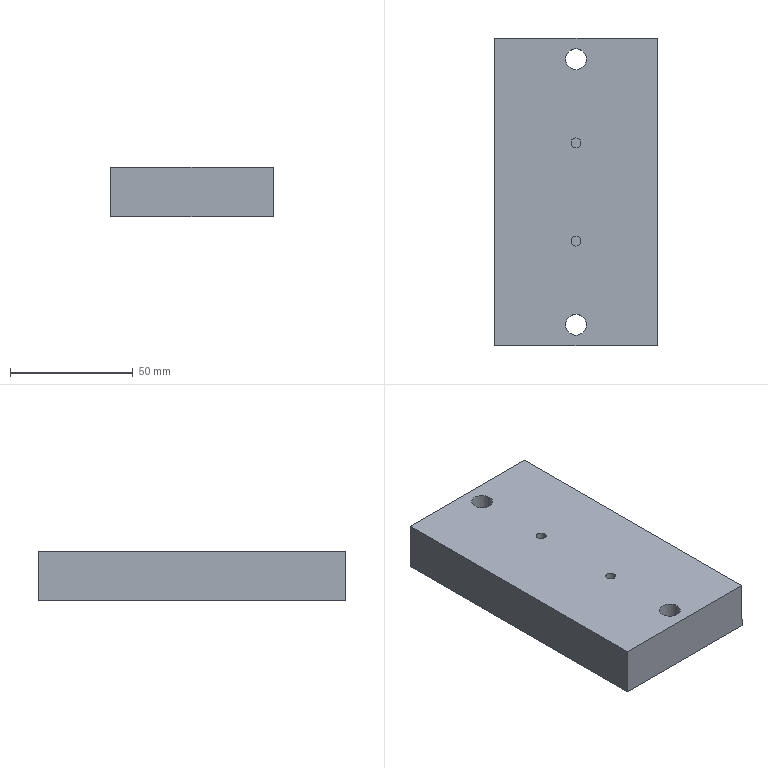NC program | NX | posted with a generic post | part box 65.936 x 125 x 20 mm
Lines 1 to 1208 of 29196:
N10 G17 G21 G94 G90
(FACE_MILLING , TOOL : D63)
N12 T01 M6
N14 G54
N16 G17 G0 G90 X86.95 Y-24.269 S4000 M3
N18 G43 Z33. H1
N20 G94 G1 Z0. F5000.
N22 X77.5 F1200.
N24 X-77.5
N26 Y24.269
N28 X77.5
N30 X86.95
N32 G0 Z33.
(FLOOR_WALL , TOOL : D63)
N34 X82.5 Y-2.101
N36 Z30.
N38 G1 Z-1.852 F5000.
N40 X74.5 F1500.
N42 X-74.5
N44 Y2.507
N46 X74.5
N48 X82.5
N50 G0 Y-2.101 Z-3.277
N52 G1 X74.5
N54 X-74.5
N56 Y2.507
N58 X74.5
N60 X82.5
N62 G0 Z30.
(FLOOR_WALL_COPY , TOOL : D63)
N64 Y-1.542
N66 G1 Z-3.427 F5000.
N68 X74.5 F1200.
N70 X-74.5
N72 Y2.402
N74 X74.5
N76 X82.5
N78 G0 Z30.
N80 M5
(PLANAR_MILL , TOOL : D16R0波刀)
N82 T02 M6
N84 G54
N86 G17 G0 G90 X-57.998 Y49.656 S5500 M3
N88 G43 Z30. H2
N90 G94 G1 Z-2.5 F5000.
N92 X-45.998 F2000.
N94 X54.35
N96 Y-41.952
N98 X46.374 Y-49.656
N100 X-46.374
N102 X-54.35 Y-41.952
N104 Y36.799
N106 Y48.799
N108 G0 X-57.998 Y49.656 Z-5.
N110 G1 X-45.998
N112 X54.35
N114 Y-41.952
N116 X46.374 Y-49.656
N118 X-46.374
N120 X-54.35 Y-41.952
N122 Y36.799
N124 Y48.799
N126 G0 X-57.998 Y49.656 Z-7.5
N128 G1 X-45.998
N130 X54.35
N132 Y-41.952
N134 X46.374 Y-49.656
N136 X-46.374
N138 X-54.35 Y-41.952
N140 Y36.799
N142 Y48.799
N144 G0 X-57.998 Y49.656 Z-10.
N146 G1 X-45.998
N148 X54.35
N150 Y-41.952
N152 X46.374 Y-49.656
N154 X-46.374
N156 X-54.35 Y-41.952
N158 Y36.799
N160 Y48.799
N162 G0 X-57.998 Y49.656 Z-12.5
N164 G1 X-45.998
N166 X54.35
N168 Y-41.952
N170 X46.374 Y-49.656
N172 X-46.374
N174 X-54.35 Y-41.952
N176 Y36.799
N178 Y48.799
N180 G0 X-57.998 Y49.656 Z-15.
N182 G1 X-45.998
N184 X54.35
N186 Y-41.952
N188 X46.374 Y-49.656
N190 X-46.374
N192 X-54.35 Y-41.952
N194 Y36.799
N196 Y48.799
N198 G0 X-57.998 Y49.656 Z-17.5
N200 G1 X-45.998
N202 X54.35
N204 Y-41.952
N206 X46.374 Y-49.656
N208 X-46.374
N210 X-54.35 Y-41.952
N212 Y36.799
N214 Y48.799
N216 G0 X-57.998 Y49.656 Z-20.
N218 G1 X-45.998
N220 X54.35
N222 Y-41.952
N224 X46.374 Y-49.656
N226 X-46.374
N228 X-54.35 Y-41.952
N230 Y36.799
N232 Y48.799
N234 G0 X-57.998 Y49.656 Z-22.5
N236 G1 X-45.998
N238 X54.35
N240 Y-41.952
N242 X46.374 Y-49.656
N244 X-46.374
N246 X-54.35 Y-41.952
N248 Y36.799
N250 Y48.799
N252 G0 X-57.998 Y49.656 Z-25.
N254 G1 X-45.998
N256 X54.35
N258 Y-41.952
N260 X46.374 Y-49.656
N262 X-46.374
N264 X-54.35 Y-41.952
N266 Y36.799
N268 Y48.799
N270 G0 X-57.998 Y49.656 Z-27.5
N272 G1 X-45.998
N274 X54.35
N276 Y-41.952
N278 X46.374 Y-49.656
N280 X-46.374
N282 X-54.35 Y-41.952
N284 Y36.799
N286 Y48.799
N288 G0 X-57.998 Y49.656 Z-28.352
N290 G1 X-45.998
N292 X54.35
N294 Y-41.952
N296 X46.374 Y-49.656
N298 X-46.374
N300 X-54.35 Y-41.952
N302 Y36.799
N304 Y48.799
N306 G0 Z30.
(PLANAR_MILL_COPY , TOOL : D16R0波刀)
N308 Z30.
N310 X58. Y-37.306
N312 G1 Z-2.335 F5000.
N314 X46. F2000.
N316 X-46.
N318 X-58.
N320 G0 Z30.
(ZLEVEL_PROFILE , TOOL : D16R0波刀)
N322 Z30.5
N324 X-56.72 Y45.12
N326 G1 Z0.203 F5000.
N328 X-46.32 F4000.
N330 X46.32
N332 X56.72
N334 G0 X56.871 Y45.544 Z-0.094
N336 G1 X46.471
N338 X-46.471
N340 X-56.871
N342 G0 Y45.967 Z-0.39
N344 G1 X-46.471
N346 X46.471
N348 X56.871
N350 G0 Y46.325 Z-0.687
N352 G1 X46.472 Y46.391
N354 X46.419
N356 X-46.472
N358 X-56.872
N360 G0 X-56.873 Y46.815 Z-0.984
N362 G1 X-46.473
N364 X46.421
N366 X46.473
N368 X56.872 Y46.751
N370 G0 Y47.184 Z-1.281
N372 G1 X46.473 Y47.239
N374 X46.429
N376 X-46.473
N378 X-56.873
N380 G0 X-56.872 Y47.663 Z-1.577
N382 G1 X-46.472
N384 X46.428
N386 X46.472 Y47.662
N388 X56.872 Y47.607
N390 G0 Y48.056 Z-1.874
N392 G1 X46.472 Y48.086
N394 X46.447
N396 X-46.472 Y48.087
N398 X-56.872
N400 G0 X-56.871 Y48.51 Z-2.171
N402 G1 X-46.471
N404 X46.471
N406 X56.871
N408 G0 Y48.934 Z-2.468
N410 G1 X46.471
N412 X-46.471
N414 X-56.871
N416 G0 X-56.682 Y49.358 Z-2.764
N418 G1 X-46.282
N420 X46.282
N422 X56.682
N424 G0 X56.299 Y49.782 Z-3.061
N426 G1 X45.899
N428 X-45.899
N430 X-56.299
N432 G0 Z30.5
(ZLEVEL_PROFILE_COPY_COPY_COPY , TOOL : D16R0波刀)
N434 X56.484 Y28.517
N436 Z30.5
N438 G1 Z0.205 F5000.
N440 X46.084 F4000.
N442 X-46.084
N444 X-56.484
N446 G0 X-56.705 Y28.323 Z-0.09
N448 G1 X-46.305 Y28.311
N450 X-45.799 Y28.31
N452 X45.799
N454 X46.305 Y28.311
N456 X56.705 Y28.323
N458 G0 X56.871 Y28.116 Z-0.385
N460 G1 X46.471 Y28.104
N462 X45.761
N464 X-46.471
N466 X-56.871
N468 G0 Y27.897 Z-0.681
N470 G1 X-46.471
N472 X45.761
N474 X46.471 Y27.898
N476 X56.871 Y27.909
N478 G0 X56.888 Y27.69 Z-0.976
N480 G1 X46.488
N482 X-46.471
N484 X-56.871
N486 G0 Y27.484 Z-1.271
N488 G1 X-46.471
N490 X45.761
N492 X46.471
N494 X56.871 Y27.496
N496 G0 X56.899 Y27.277 Z-1.566
N498 G1 X46.499
N500 X-46.47
N502 X-56.871
N504 G0 Y27.071 Z-1.861
N506 G1 X-46.471 Y27.07
N508 X45.761
N510 X46.471 Y27.071
N512 X56.871 Y27.082
N514 G0 X56.899 Y26.864 Z-2.156
N516 G1 X46.499
N518 X-46.467
N520 X-46.471
N522 X-56.871 Y26.868
N524 G0 Y26.662 Z-2.451
N526 G1 X-46.471 Y26.657
N528 X-46.467
N530 X46.504
N532 X56.904
N534 G0 X56.902 Y26.45 Z-2.747
N536 G1 X46.502
N538 X-46.465
N540 X-56.865
N542 G0 X-56.561 Y26.256 Z-3.042
N544 G1 X-46.161 Y26.244
N546 X-45.799
N548 X45.799
N550 X46.161
N552 X56.561 Y26.256
N554 G0 X56.374 Y26.038 Z-3.337
N556 G1 X45.974
N558 X-45.974
N560 X-56.374
N562 G0 Z30.5
(ZLEVEL_PROFILE_COPY , TOOL : D16R0波刀)
N564 X56.709 Y-45.181
N566 Z27.965
N568 G1 Z-2.313 F5000.
N570 X46.309 F4000.
N572 X-46.309
N574 X-56.709
N576 G0 X-56.871 Y-45.63 Z-2.592
N578 G1 X-46.471 Y-45.663
N580 X-46.445
N582 X46.471
N584 X56.871
N586 G0 Y-46.146 Z-2.871
N588 G1 X46.471
N590 X-46.422
N592 X-46.471 Y-46.145
N594 X-56.871 Y-46.084
N596 G0 Y-46.595 Z-3.149
N598 G1 X-46.471 Y-46.628
N600 X-46.445
N602 X46.471
N604 X56.871
N606 G0 Y-47.111 Z-3.428
N608 G1 X46.471
N610 X-46.445
N612 X-46.471
N614 X-56.871 Y-47.078
N616 G0 Y-47.593 Z-3.706
N618 G1 X-46.471
N620 X46.471
N622 X56.871
N624 G0 Y-48.076 Z-3.985
N626 G1 X46.471
N628 X-46.464
N630 X-46.471
N632 X-56.871 Y-48.067
N634 G0 Y-48.492 Z-4.263
N636 G1 X-46.471 Y-48.558
N638 X-46.419
N640 X46.471
N642 X56.871
N644 G0 Y-49.041 Z-4.542
N646 G1 X46.471
N648 X-46.471
N650 X-56.871
N652 G0 X-56.618 Y-49.523 Z-4.821
N654 G1 X-46.218
N656 X46.218
N658 X56.618
N660 G0 Z27.965
(ZLEVEL_PROFILE_COPY_COPY , TOOL : D16R0波刀)
N662 X-56.871 Y-28.436
N664 G1 Z-2.305 F5000.
N666 X-46.471 Y-28.371 F3000.
N668 X-46.42
N670 X46.42
N672 X46.471
N674 X56.871 Y-28.436
N676 G0 X56.872 Y-27.362 Z-2.576
N678 G1 X46.472
N680 X-46.472
N682 X-56.872
N684 G0 X-56.871 Y-26.411 Z-2.846
N686 G1 X-46.471 Y-26.353
N688 X-46.426
N690 X46.426
N692 X46.471
N694 X56.871 Y-26.411
N696 G0 X56.517 Y-25.356 Z-3.116
N698 G1 X46.117 Y-25.344
N700 X45.799 Y-25.343
N702 X-45.799
N704 X-46.117 Y-25.344
N706 X-56.517 Y-25.356
N708 G0 Z27.965
N710 M5
(PLANAR_MILL_COPY_COPY , TOOL : D8R0)
N712 T03 M6
N714 G54
N716 G17 G0 G90 X51.2 Y30.401 S4500 M3
N718 G43 Z26.583 H3
N720 G94 G1 Z-3.417 F5000.
N722 X46. F1000.
N724 X-46.
N726 X-51.2
N728 G0 Z26.583
N730 Y-29.535
N732 G1 Z-3.417 F5000.
N734 X-46. F1000.
N736 X46.
N738 X51.2
N740 G0 Z26.583
(PLANAR_MILL_COPY_2 , TOOL : D8R0)
N742 Z30.
N744 X-51.999 Y45.306
N746 G1 Z-15. F5000.
N748 X-45.999 F800.
N750 X50.
N752 Y-40.106
N754 X44.616 Y-45.306
N756 X-44.616
N758 X-50. Y-40.106
N760 Y36.799
N762 Y43.999
N764 G0 X-51.999 Y45.306 Z-28.352
N766 G1 X-45.999
N768 X50.
N770 Y-40.106
N772 X44.616 Y-45.306
N774 X-44.616
N776 X-50. Y-40.106
N778 Y36.799
N780 Y43.999
N782 G0 Z30.
N784 M5
(FIXED_CONTOUR , TOOL : D4R0.5)
N786 T04 M6
N788 G54
N790 G17 G0 G90 X-48. Y40.587 S6000 M3
N792 G43 Z30. H4
N794 G94 G1 Z-0.09 F5000.
N796 G3 X-46. Y38.587 R2. F3000.
N798 G1 X46.
N800 Y38.663 Z-0.143
N802 X-46.
N804 Y38.738 Z-0.196
N806 X46.
N808 Y38.813 Z-0.248
N810 X-46.
N812 Y38.888 Z-0.301
N814 X46.
N816 Y38.963 Z-0.353
N818 X-46.
N820 Y39.038 Z-0.406
N822 X46.
N824 Y39.113 Z-0.458
N826 X-46.
N828 Y39.188 Z-0.511
N830 X46.
N832 Y39.263 Z-0.564
N834 X-46.
N836 Y39.338 Z-0.616
N838 X46.
N840 Y39.413 Z-0.669
N842 X-46.
N844 Y39.489 Z-0.721
N846 X46.
N848 Y39.564 Z-0.774
N850 X-46.
N852 Y39.639 Z-0.827
N854 X46.
N856 Y39.714 Z-0.879
N858 X-46.
N860 Y39.789 Z-0.932
N862 X46.
N864 Y39.864 Z-0.984
N866 X-46.
N868 Y39.939 Z-1.037
N870 X46.
N872 Y40.014 Z-1.089
N874 X-46.
N876 Y40.089 Z-1.142
N878 X46.
N880 Y40.164 Z-1.195
N882 X-46.
N884 Y40.239 Z-1.247
N886 X46.
N888 Y40.314 Z-1.3
N890 X-46.
N892 Y40.39 Z-1.352
N894 X46.
N896 Y40.465 Z-1.405
N898 X-46.
N900 Y40.54 Z-1.457
N902 X46.
N904 Y40.615 Z-1.51
N906 X-46.
N908 Y40.69 Z-1.563
N910 X46.
N912 Y40.765 Z-1.615
N914 X-46.
N916 Y40.84 Z-1.668
N918 X46.
N920 Y40.915 Z-1.72
N922 X-46.
N924 Y40.99 Z-1.773
N926 X46.
N928 Y41.065 Z-1.825
N930 X-46.
N932 Y41.14 Z-1.878
N934 X46.
N936 Y41.216 Z-1.931
N938 X-46.
N940 Y41.291 Z-1.983
N942 X46.
N944 Y41.366 Z-2.036
N946 X-46.
N948 Y41.441 Z-2.088
N950 X46.
N952 Y41.516 Z-2.141
N954 X-46.
N956 Y41.591 Z-2.194
N958 X46.
N960 Y41.666 Z-2.246
N962 X-46.
N964 Y41.741 Z-2.299
N966 X46.
N968 Y41.816 Z-2.351
N970 X-46.
N972 Y41.891 Z-2.404
N974 X46.
N976 Y41.966 Z-2.456
N978 X-46.
N980 Y42.042 Z-2.509
N982 X46.
N984 Y42.117 Z-2.562
N986 X-46.
N988 Y42.192 Z-2.614
N990 X46.
N992 Y42.267 Z-2.667
N994 X-46.
N996 Y42.342 Z-2.719
N998 X46.
N1000 Y42.417 Z-2.772
N1002 X-46.
N1004 Y42.492 Z-2.824
N1006 X46.
N1008 Y42.567 Z-2.877
N1010 X-46.
N1012 Y42.642 Z-2.93
N1014 X46.
N1016 Y42.717 Z-2.982
N1018 X-46.
N1020 Y42.792 Z-3.035
N1022 X46.
N1024 Y42.868 Z-3.087
N1026 X-46.
N1028 Y42.943 Z-3.14
N1030 X46.
N1032 Y43.018 Z-3.193
N1034 X-46.
N1036 Y43.093 Z-3.245
N1038 X46.
N1040 G3 X48. Y45.093 R2.
N1042 G0 Z30.
(ZLEVEL_PROFILE_1 , TOOL : D4R0.5)
N1044 X48.6 Y34.874
N1046 G1 Z-0.237 F5000.
N1048 X46. F2500.
N1050 X-46.
N1052 X-48.6
N1054 G0 Y34.819 Z-0.316
N1056 G1 X-46.
N1058 X46.
N1060 X48.6
N1062 G0 Y34.764 Z-0.395
N1064 G1 X46.
N1066 X-46.
N1068 X-48.6
N1070 G0 Y34.708 Z-0.474
N1072 G1 X-46.
N1074 X46.
N1076 X48.6
N1078 G0 Y34.653 Z-0.553
N1080 G1 X46.
N1082 X-46.
N1084 X-48.6
N1086 G0 Y34.597 Z-0.633
N1088 G1 X-46.
N1090 X46.
N1092 X48.6
N1094 G0 Y34.542 Z-0.712
N1096 G1 X46.
N1098 X-46.
N1100 X-48.6
N1102 G0 Y34.487 Z-0.791
N1104 G1 X-46.
N1106 X46.
N1108 X48.6
N1110 G0 Y34.431 Z-0.87
N1112 G1 X46.
N1114 X-46.
N1116 X-48.6
N1118 G0 Y34.376 Z-0.949
N1120 G1 X-46.
N1122 X46.
N1124 X48.6
N1126 G0 Y34.321 Z-1.028
N1128 G1 X46.
N1130 X-46.
N1132 X-48.6
N1134 G0 Y34.265 Z-1.107
N1136 G1 X-46.
N1138 X46.
N1140 X48.6
N1142 G0 Y34.21 Z-1.186
N1144 G1 X46.
N1146 X-46.
N1148 X-48.6
N1150 G0 Y34.155 Z-1.265
N1152 G1 X-46.
N1154 X46.
N1156 X48.6
N1158 G0 Y34.099 Z-1.344
N1160 G1 X46.
N1162 X-46.
N1164 X-48.6
N1166 G0 Y34.044 Z-1.423
N1168 G1 X-46.
N1170 X46.
N1172 X48.6
N1174 G0 Y33.988 Z-1.502
N1176 G1 X46.
N1178 X-46.
N1180 X-48.6
N1182 G0 Y33.933 Z-1.581
N1184 G1 X-46.
N1186 X46.
N1188 X48.6
N1190 G0 Y33.878 Z-1.66
N1192 G1 X46.
N1194 X-46.
N1196 X-48.6
N1198 G0 Y33.822 Z-1.74
N1200 G1 X-46.
N1202 X46.
N1204 X48.6
N1206 G0 Y33.767 Z-1.819
N1208 G1 X46.
N1210 X-46.
N1212 X-48.6
N1214 G0 Y33.712 Z-1.898
N1216 G1 X-46.
N1218 X46.
N1220 X48.6
N1222 G0 Y33.656 Z-1.977
N1224 G1 X46.
N1226 X-46.
N1228 X-48.6
N1230 G0 Y33.601 Z-2.056
N1232 G1 X-46.
N1234 X46.
N1236 X48.6
N1238 G0 Y33.546 Z-2.135
N1240 G1 X46.
N1242 X-46.
N1244 X-48.6
N1246 G0 Y33.49 Z-2.214
N1248 G1 X-46.
N1250 X46.
N1252 X48.6
N1254 G0 Y33.435 Z-2.293
N1256 G1 X46.
N1258 X-46.
N1260 X-48.6
N1262 G0 Y33.379 Z-2.372
N1264 G1 X-46.
N1266 X46.
N1268 X48.6
N1270 G0 Y33.324 Z-2.451
N1272 G1 X46.
N1274 X-46.
N1276 X-48.6
N1278 G0 Y33.269 Z-2.53
N1280 G1 X-46.
N1282 X46.
N1284 X48.6
N1286 G0 Y33.213 Z-2.609
N1288 G1 X46.
N1290 X-46.
N1292 X-48.6
N1294 G0 Y33.158 Z-2.688
N1296 G1 X-46.
N1298 X46.
N1300 X48.6
N1302 G0 Y33.103 Z-2.767
N1304 G1 X46.
N1306 X-46.
N1308 X-48.6
N1310 G0 Y33.047 Z-2.847
N1312 G1 X-46.
N1314 X46.
N1316 X48.6
N1318 G0 Y32.992 Z-2.926
N1320 G1 X46.
N1322 X-46.
N1324 X-48.6
N1326 G0 Y32.936 Z-3.005
N1328 G1 X-46.
N1330 X46.
N1332 X48.6
N1334 G0 Y32.881 Z-3.084
N1336 G1 X46.
N1338 X-46.
N1340 X-48.6
N1342 G0 Y32.826 Z-3.163
N1344 G1 X-46.
N1346 X46.
N1348 X48.6
N1350 G0 Y32.77 Z-3.242
N1352 G1 X46.
N1354 X-46.
N1356 X-48.6
N1358 G0 Y32.715 Z-3.321
N1360 G1 X-46.
N1362 X46.
N1364 X48.6
N1366 G0 Y32.66 Z-3.4
N1368 G1 X46.
N1370 X-46.
N1372 X-48.6
N1374 G0 Z30.
(ZLEVEL_PROFILE_1_COPY , TOOL : D4R0.5)
N1376 X-48.653 Y-35.529
N1378 Z27.665
N1380 G1 Z-2.515 F5000.
N1382 X-46.057 Y-35.378 F2000.
N1384 X-45.987 Y-35.374
N1386 X45.987
N1388 X46.057 Y-35.378
N1390 X48.653 Y-35.529
N1392 G0 X48.785 Y-35.3 Z-2.535
N1394 G1 X46.185 Y-35.299
N1396 X45.987
N1398 X-46.185
N1400 X-48.785
N1402 G0 Y-35.225 Z-2.555
N1404 G1 X-46.185
N1406 X45.987
N1408 X46.185
N1410 X48.785
N1412 G0 Y-35.211 Z-2.575
N1414 G1 X46.185 Y-35.151
N1416 X46.144 Y-35.15
N1418 X-46.146
N1420 X-46.185
N1422 X-48.785 Y-35.209
N1424 G0 Y-35.075 Z-2.595
N1426 G1 X-46.185
N1428 X45.987
N1430 X46.185
N1432 X48.785
N1434 G0 Y-35.001 Z-2.615
N1436 G1 X46.185
N1438 X-46.185
N1440 X-48.785
N1442 G0 Y-34.926 Z-2.635
N1444 G1 X-46.185
N1446 X46.185
N1448 X48.785
N1450 G0 Y-34.883 Z-2.655
N1452 G1 X46.185 Y-34.852
N1454 X46.165 Y-34.851
N1456 X-46.164
N1458 X-46.185 Y-34.852
N1460 X-48.785 Y-34.883
N1462 G0 Y-34.777 Z-2.675
N1464 G1 X-46.185
N1466 X46.159
N1468 X46.185
N1470 X48.785 Y-34.816
N1472 G0 Y-34.761 Z-2.695
N1474 G1 X46.185 Y-34.703
N1476 X46.146 Y-34.702
N1478 X-46.146
N1480 X-46.185 Y-34.703
N1482 X-48.785 Y-34.761
N1484 G0 Y-34.687 Z-2.715
N1486 G1 X-46.185 Y-34.628
N1488 X-46.145
N1490 X46.145
N1492 X46.185
N1494 X48.785 Y-34.688
N1496 G0 Y-34.611 Z-2.735
N1498 G1 X46.185 Y-34.553
N1500 X46.146
N1502 X-46.146
N1504 X-46.185
N1506 X-48.785 Y-34.611
N1508 G0 Y-34.541 Z-2.755
N1510 G1 X-46.185 Y-34.479
N1512 X-46.143 Y-34.478
N1514 X46.144
N1516 X46.185 Y-34.479
N1518 X48.785 Y-34.54
N1520 G0 Y-34.463 Z-2.775
N1522 G1 X46.185 Y-34.404
N1524 X46.145
N1526 X-46.146
N1528 X-46.185
N1530 X-48.785 Y-34.462
N1532 G0 Y-34.387 Z-2.795
N1534 G1 X-46.185 Y-34.329
N1536 X-46.146
N1538 X46.147
N1540 X46.185
N1542 X48.785 Y-34.386
N1544 G0 Y-34.254 Z-2.815
N1546 G1 X46.185
N1548 X-46.185
N1550 X-48.785 Y-34.255
N1552 G0 Y-34.18 Z-2.835
N1554 G1 X-46.185
N1556 X46.185
N1558 X48.785
N1560 G0 Y-34.105 Z-2.855
N1562 G1 X46.185
N1564 X-46.185
N1566 X-48.785
N1568 G0 X-48.786 Y-34.03 Z-2.875
N1570 G1 X-46.186
N1572 X46.186
N1574 X48.786
N1576 G0 Y-33.956 Z-2.895
N1578 G1 X46.186
N1580 X-46.186
N1582 X-48.786
N1584 G0 Y-33.881 Z-2.915
N1586 G1 X-46.186
N1588 X46.186
N1590 X48.786
N1592 G0 Y-33.806 Z-2.935
N1594 G1 X46.186
N1596 X-46.186
N1598 X-48.786
N1600 G0 Y-33.732 Z-2.955
N1602 G1 X-46.186
N1604 X46.186
N1606 X48.786
N1608 G0 Y-33.657 Z-2.975
N1610 G1 X46.186
N1612 X-46.186
N1614 X-48.786
N1616 G0 Y-33.583 Z-2.995
N1618 G1 X-46.186
N1620 X46.186
N1622 X48.786
N1624 G0 Y-33.508 Z-3.015
N1626 G1 X46.186
N1628 X-46.186 Y-33.52
N1630 X-48.786
N1632 G0 Y-33.494 Z-3.035
N1634 G1 X-46.186 Y-33.434
N1636 X-46.145 Y-33.433
N1638 X46.146
N1640 X46.186 Y-33.434
N1642 X48.786 Y-33.493
N1644 G0 Y-33.416 Z-3.055
N1646 G1 X46.186 Y-33.359
N1648 X46.148
N1650 X-46.148
N1652 X-46.186
N1654 X-48.786 Y-33.416
N1656 G0 Y-33.346 Z-3.075
N1658 G1 X-46.186 Y-33.285
N1660 X-46.144 Y-33.284
N1662 X46.144
N1664 X46.186 Y-33.285
N1666 X48.785 Y-33.346
N1668 G0 X48.786 Y-33.269 Z-3.095
N1670 G1 X46.186 Y-33.21
N1672 X46.146 Y-33.209
N1674 X-46.146
N1676 X-46.186 Y-33.21
N1678 X-48.786 Y-33.269
N1680 G0 Y-33.192 Z-3.115
N1682 G1 X-46.186 Y-33.135
N1684 X-46.147
N1686 X46.147
N1688 X46.186
N1690 X48.786 Y-33.193
N1692 G0 X48.785 Y-33.121 Z-3.135
N1694 G1 X46.186 Y-33.061
N1696 X46.145 Y-33.06
N1698 X-46.146
N1700 X-46.186 Y-33.061
N1702 X-48.785 Y-33.12
N1704 G0 X-48.786 Y-32.985 Z-3.155
N1706 G1 X-46.186
N1708 X46.146
N1710 X46.186 Y-32.986
N1712 X48.785 Y-33.044
N1714 G0 Y-32.911 Z-3.175
N1716 G1 X46.185
N1718 X-46.185
N1720 X-48.785
N1722 G0 Y-32.836 Z-3.195
N1724 G1 X-46.185
N1726 X46.185
N1728 X48.785
N1730 G0 Y-32.762 Z-3.215
N1732 G1 X46.185
N1734 X-46.185
N1736 X-48.785
N1738 G0 Y-32.687 Z-3.235
N1740 G1 X-46.185
N1742 X46.185
N1744 X48.785
N1746 G0 Y-32.612 Z-3.255
N1748 G1 X46.185
N1750 X-46.185
N1752 X-48.785
N1754 G0 Y-32.538 Z-3.275
N1756 G1 X-46.185
N1758 X46.185
N1760 X48.785
N1762 G0 Y-32.497 Z-3.295
N1764 G1 X46.185 Y-32.463
N1766 X46.163
N1768 X-46.163
N1770 X-46.185
N1772 X-48.785 Y-32.497
N1774 G0 Y-32.388 Z-3.315
N1776 G1 X-46.185
N1778 X46.185
N1780 X48.785
N1782 G0 Y-32.314 Z-3.335
N1784 G1 X46.185
N1786 X-46.185
N1788 X-48.785
N1790 G0 Y-32.298 Z-3.355
N1792 G1 X-46.185 Y-32.239
N1794 X-46.145
N1796 X46.185
N1798 X48.785
N1800 G0 Y-32.19 Z-3.375
N1802 G1 X46.185 Y-32.164
N1804 X46.169
N1806 X-46.185
N1808 X-48.785
N1810 G0 Y-32.09 Z-3.395
N1812 G1 X-46.185
N1814 X46.185
N1816 X48.785
N1818 G0 Z27.665
(FIXED_CONTOUR_COPY , TOOL : D4R0.5)
N1820 X-48. Y-40.615
N1822 Z27.465
N1824 G1 Z-2.602 F5000.
N1826 G2 X-46. Y-38.615 R2. F2500.
N1828 G1 X46.
N1830 Y-38.706 Z-2.654
N1832 X-46.
N1834 Y-38.797 Z-2.707
N1836 X46.
N1838 Y-38.888 Z-2.759
N1840 X-46.
N1842 Y-38.978 Z-2.812
N1844 X46.
N1846 Y-39.069 Z-2.864
N1848 X-46.
N1850 Y-39.16 Z-2.916
N1852 X46.
N1854 Y-39.251 Z-2.969
N1856 X-46.
N1858 Y-39.342 Z-3.021
N1860 X46.
N1862 Y-39.432 Z-3.074
N1864 X-46.
N1866 Y-39.523 Z-3.126
N1868 X46.
N1870 Y-39.614 Z-3.179
N1872 X-46.
N1874 Y-39.705 Z-3.231
N1876 X46.
N1878 Y-39.796 Z-3.283
N1880 X-46.
N1882 Y-39.886 Z-3.336
N1884 X46.
N1886 Y-39.977 Z-3.388
N1888 X-46.
N1890 Y-40.068 Z-3.441
N1892 X46.
N1894 Y-40.159 Z-3.493
N1896 X-46.
N1898 Y-40.25 Z-3.546
N1900 X46.
N1902 Y-40.34 Z-3.598
N1904 X-46.
N1906 Y-40.431 Z-3.65
N1908 X46.
N1910 Y-40.522 Z-3.703
N1912 X-46.
N1914 Y-40.613 Z-3.755
N1916 X46.
N1918 Y-40.704 Z-3.808
N1920 X-46.
N1922 Y-40.794 Z-3.86
N1924 X46.
N1926 Y-40.885 Z-3.913
N1928 X-46.
N1930 Y-40.976 Z-3.965
N1932 X46.
N1934 Y-41.067 Z-4.017
N1936 X-46.
N1938 Y-41.158 Z-4.07
N1940 X46.
N1942 Y-41.248 Z-4.122
N1944 X-46.
N1946 Y-41.339 Z-4.175
N1948 X46.
N1950 Y-41.43 Z-4.227
N1952 X-46.
N1954 Y-41.521 Z-4.28
N1956 X46.
N1958 Y-41.612 Z-4.332
N1960 X-46.
N1962 Y-41.703 Z-4.384
N1964 X46.
N1966 Y-41.793 Z-4.437
N1968 X-46.
N1970 Y-41.884 Z-4.489
N1972 X46.
N1974 Y-41.975 Z-4.542
N1976 X-46.
N1978 Y-42.066 Z-4.594
N1980 X46.
N1982 Y-42.157 Z-4.647
N1984 X-46.
N1986 Y-42.247 Z-4.699
N1988 X46.
N1990 Y-42.338 Z-4.751
N1992 X-46.
N1994 Y-42.429 Z-4.804
N1996 X46.
N1998 Y-42.52 Z-4.856
N2000 X-46.
N2002 Y-42.611 Z-4.909
N2004 X46.
N2006 Y-42.701 Z-4.961
N2008 X-46.
N2010 Y-42.792 Z-5.014
N2012 X46.
N2014 Y-42.883 Z-5.066
N2016 X-46.
N2018 Y-42.974 Z-5.118
N2020 X46.
N2022 Y-43.065 Z-5.171
N2024 X-46.
N2026 Y-43.155 Z-5.223
N2028 X46.
N2030 G2 X48. Y-45.155 R2.
N2032 G0 Z27.465
(FIXED_CONTOUR_COPY_COPY , TOOL : D4R0.5)
N2034 X-48. Y-44.522
N2036 Z25.344
N2038 G1 Z-5.027 F5000.
N2040 G2 X-46. Y-42.522 R2. F3000.
N2042 G1 X46.
N2044 Y-42.538 Z-5.084
N2046 X-46.
N2048 Y-42.553 Z-5.141
N2050 X46.
N2052 Y-42.568 Z-5.198
N2054 X-46.
N2056 Y-42.584 Z-5.256
N2058 X46.
N2060 Y-42.599 Z-5.313
N2062 X-46.
N2064 Y-42.614 Z-5.37
N2066 X46.
N2068 Y-42.63 Z-5.427
N2070 X-46.
N2072 Y-42.645 Z-5.485
N2074 X46.
N2076 Y-42.66 Z-5.542
N2078 X-46.
N2080 Y-42.676 Z-5.599
N2082 X46.
N2084 Y-42.691 Z-5.656
N2086 X-46.
N2088 Y-42.706 Z-5.713
N2090 X46.
N2092 Y-42.722 Z-5.771
N2094 X-46.
N2096 Y-42.737 Z-5.828
N2098 X46.
N2100 Y-42.752 Z-5.885
N2102 X-46.
N2104 Y-42.768 Z-5.942
N2106 X46.
N2108 Y-42.783 Z-6.
N2110 X-46.
N2112 Y-42.798 Z-6.057
N2114 X46.
N2116 Y-42.814 Z-6.114
N2118 X-46.
N2120 Y-42.829 Z-6.171
N2122 X46.
N2124 Y-42.844 Z-6.228
N2126 X-46.
N2128 Y-42.86 Z-6.286
N2130 X46.
N2132 Y-42.875 Z-6.343
N2134 X-46.
N2136 Y-42.89 Z-6.4
N2138 X46.
N2140 Y-42.906 Z-6.457
N2142 X-46.
N2144 Y-42.921 Z-6.515
N2146 X46.
N2148 Y-42.936 Z-6.572
N2150 X-46.
N2152 Y-42.952 Z-6.629
N2154 X46.
N2156 Y-42.967 Z-6.686
N2158 X-46.
N2160 Y-42.982 Z-6.743
N2162 X46.
N2164 Y-42.998 Z-6.801
N2166 X-46.
N2168 Y-43.013 Z-6.858
N2170 X46.
N2172 Y-43.028 Z-6.915
N2174 X-46.
N2176 Y-43.044 Z-6.972
N2178 X46.
N2180 Y-43.059 Z-7.03
N2182 X-46.
N2184 Y-43.074 Z-7.087
N2186 X46.
N2188 Y-43.09 Z-7.144
N2190 X-46.
N2192 Y-43.105 Z-7.201
N2194 X46.
N2196 Y-43.12 Z-7.258
N2198 X-46.
N2200 Y-43.136 Z-7.316
N2202 X46.
N2204 Y-43.151 Z-7.373
N2206 X-46.
N2208 Y-43.166 Z-7.43
N2210 X46.
N2212 Y-43.182 Z-7.487
N2214 X-46.
N2216 Y-43.197 Z-7.545
N2218 X46.
N2220 Y-43.212 Z-7.602
N2222 X-46.
N2224 Y-43.228 Z-7.659
N2226 X46.
N2228 Y-43.243 Z-7.716
N2230 X-46.
N2232 Y-43.258 Z-7.773
N2234 X46.
N2236 Y-43.274 Z-7.831
N2238 X-46.
N2240 Y-43.289 Z-7.888
N2242 X46.
N2244 G2 X48. Y-45.289 R2.
N2246 G0 Z25.344
N2248 M5
(DRILLING , TOOL : DK-D10)
N2250 T05 M6
N2252 G54
N2254 G17 G0 G90 X-30. Y-5.802 S2000 M3
N2256 G43 Z26.573 H5
N2258 G94 G81 G99 Z-5.627 F200. R-1.927
N2260 G0 Z26.573
N2262 G81 X30. Z-5.627 R-1.927
N2264 G0 Z26.573
N2266 G80
N2268 G0 X30. Y-5.802 Z26.573
(DRILLING_COPY_1 , TOOL : DK-D10)
N2270 X-30. Y4.198
N2272 G81 Z-7.527 F200. R-1.927
N2274 G0 Z26.573
N2276 G81 X30. Z-7.527 R-1.927
N2278 G0 Z26.573
N2280 G80
N2282 G0 X30. Y4.198 Z26.573
N2284 M5
(DRILLING_COPY , TOOL : D6.8钻头)
N2286 T06 M6
N2288 G54
N2290 G17 G0 G90 X30. Y4.198 S2000 M3
N2292 G43 Z26.573 H6
N2294 G94 G83 G99 Z-15.427 F200. Q3. R-1.927
N2296 G0 Z26.573
N2298 G83 X-30. Z-15.427 Q3. R-1.927
N2300 G0 Z26.573
N2302 G80
N2304 G0 X-30. Y4.198 Z26.573
N2306 M5